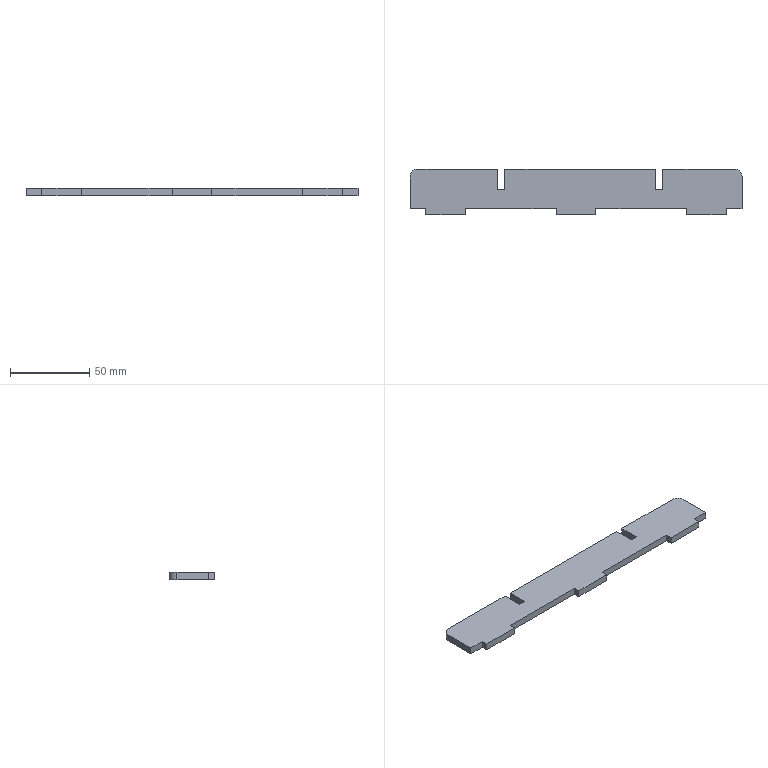Part | SolidWorks | features FlatPattern 1, SMBaseFlange 1, SheetMetal 1 | 1 solid | 28 faces | box 210 x 29 x 4.5 mm | volume 24400 mm3 | plane 26 | cylinder 2 | commonest cylinder face diameters 10 x2
STEP:
#1=CARTESIAN_POINT('',(71.625,-115.747,0.));
#2=VERTEX_POINT('',#1);
#3=CARTESIAN_POINT('',(71.625,-95.747,0.));
#4=VERTEX_POINT('',#3);
#5=CARTESIAN_POINT('',(71.625,-115.747,0.));
#6=DIRECTION('',(0.,1.,0.));
#7=VECTOR('',#6,1000.);
#8=LINE('',#5,#7);
#9=EDGE_CURVE('',#2,#4,#8,.T.);
#10=ORIENTED_EDGE('',*,*,#9,.F.);
#11=CARTESIAN_POINT('',(71.625,-115.747,-4.5));
#12=VERTEX_POINT('',#11);
#13=CARTESIAN_POINT('',(71.625,-115.747,-4.5));
#14=DIRECTION('',(0.,0.,1.));
#15=VECTOR('',#14,1000.);
#16=LINE('',#13,#15);
#17=EDGE_CURVE('',#12,#2,#16,.T.);
#18=ORIENTED_EDGE('',*,*,#17,.F.);
#19=CARTESIAN_POINT('',(71.625,-95.747,-4.5));
#20=VERTEX_POINT('',#19);
#21=CARTESIAN_POINT('',(71.625,-115.747,-4.5));
#22=DIRECTION('',(0.,1.,0.));
#23=VECTOR('',#22,1000.);
#24=LINE('',#21,#23);
#25=EDGE_CURVE('',#12,#20,#24,.T.);
#26=ORIENTED_EDGE('',*,*,#25,.T.);
#27=CARTESIAN_POINT('',(71.625,-95.747,-4.5));
#28=DIRECTION('',(0.,0.,1.));
#29=VECTOR('',#28,1000.);
#30=LINE('',#27,#29);
#31=EDGE_CURVE('',#20,#4,#30,.T.);
#32=ORIENTED_EDGE('',*,*,#31,.T.);
#33=EDGE_LOOP('',(#10,#18,#26,#32));
#34=FACE_OUTER_BOUND('',#33,.T.);
#35=CARTESIAN_POINT('',(71.625,-115.747,-4.5));
#36=DIRECTION('',(1.,0.,0.));
#37=DIRECTION('',(0.,0.,-1.));
#38=AXIS2_PLACEMENT_3D('',#35,#36,#37);
#39=PLANE('',#38);
#40=ADVANCED_FACE('',(#34),#39,.T.);
#41=CARTESIAN_POINT('',(61.625,-115.747,0.));
#42=VERTEX_POINT('',#41);
#43=CARTESIAN_POINT('',(71.625,-115.747,0.));
#44=DIRECTION('',(1.,0.,0.));
#45=VECTOR('',#44,1000.);
#46=LINE('',#43,#45);
#47=EDGE_CURVE('',#42,#2,#46,.T.);
#48=ORIENTED_EDGE('',*,*,#47,.F.);
#49=CARTESIAN_POINT('',(61.625,-115.747,-4.5));
#50=VERTEX_POINT('',#49);
#51=CARTESIAN_POINT('',(61.625,-115.747,-4.5));
#52=DIRECTION('',(0.,0.,1.));
#53=VECTOR('',#52,1000.);
#54=LINE('',#51,#53);
#55=EDGE_CURVE('',#50,#42,#54,.T.);
#56=ORIENTED_EDGE('',*,*,#55,.F.);
#57=CARTESIAN_POINT('',(71.625,-115.747,-4.5));
#58=DIRECTION('',(1.,0.,0.));
#59=VECTOR('',#58,1000.);
#60=LINE('',#57,#59);
#61=EDGE_CURVE('',#50,#12,#60,.T.);
#62=ORIENTED_EDGE('',*,*,#61,.T.);
#63=ORIENTED_EDGE('',*,*,#17,.T.);
#64=EDGE_LOOP('',(#48,#56,#62,#63));
#65=FACE_OUTER_BOUND('',#64,.T.);
#66=CARTESIAN_POINT('',(71.625,-115.747,-4.5));
#67=DIRECTION('',(0.,-1.,0.));
#68=DIRECTION('',(0.,0.,-1.));
#69=AXIS2_PLACEMENT_3D('',#66,#67,#68);
#70=PLANE('',#69);
#71=ADVANCED_FACE('',(#65),#70,.T.);
#72=CARTESIAN_POINT('',(61.625,-119.747,0.));
#73=VERTEX_POINT('',#72);
#74=CARTESIAN_POINT('',(61.625,-115.747,0.));
#75=DIRECTION('',(0.,1.,0.));
#76=VECTOR('',#75,1000.);
#77=LINE('',#74,#76);
#78=EDGE_CURVE('',#73,#42,#77,.T.);
#79=ORIENTED_EDGE('',*,*,#78,.F.);
#80=CARTESIAN_POINT('',(61.625,-119.747,-4.5));
#81=VERTEX_POINT('',#80);
#82=CARTESIAN_POINT('',(61.625,-119.747,-4.5));
#83=DIRECTION('',(0.,0.,1.));
#84=VECTOR('',#83,1000.);
#85=LINE('',#82,#84);
#86=EDGE_CURVE('',#81,#73,#85,.T.);
#87=ORIENTED_EDGE('',*,*,#86,.F.);
#88=CARTESIAN_POINT('',(61.625,-115.747,-4.5));
#89=DIRECTION('',(0.,1.,0.));
#90=VECTOR('',#89,1000.);
#91=LINE('',#88,#90);
#92=EDGE_CURVE('',#81,#50,#91,.T.);
#93=ORIENTED_EDGE('',*,*,#92,.T.);
#94=ORIENTED_EDGE('',*,*,#55,.T.);
#95=EDGE_LOOP('',(#79,#87,#93,#94));
#96=FACE_OUTER_BOUND('',#95,.T.);
#97=CARTESIAN_POINT('',(61.625,-115.747,-4.5));
#98=DIRECTION('',(1.,0.,0.));
#99=DIRECTION('',(0.,0.,-1.));
#100=AXIS2_PLACEMENT_3D('',#97,#98,#99);
#101=PLANE('',#100);
#102=ADVANCED_FACE('',(#96),#101,.T.);
#103=CARTESIAN_POINT('',(36.625,-119.747,0.));
#104=VERTEX_POINT('',#103);
#105=CARTESIAN_POINT('',(61.625,-119.747,0.));
#106=DIRECTION('',(1.,0.,0.));
#107=VECTOR('',#106,1000.);
#108=LINE('',#105,#107);
#109=EDGE_CURVE('',#104,#73,#108,.T.);
#110=ORIENTED_EDGE('',*,*,#109,.F.);
#111=CARTESIAN_POINT('',(36.625,-119.747,-4.5));
#112=VERTEX_POINT('',#111);
#113=CARTESIAN_POINT('',(36.625,-119.747,-4.5));
#114=DIRECTION('',(0.,0.,1.));
#115=VECTOR('',#114,1000.);
#116=LINE('',#113,#115);
#117=EDGE_CURVE('',#112,#104,#116,.T.);
#118=ORIENTED_EDGE('',*,*,#117,.F.);
#119=CARTESIAN_POINT('',(61.625,-119.747,-4.5));
#120=DIRECTION('',(1.,0.,0.));
#121=VECTOR('',#120,1000.);
#122=LINE('',#119,#121);
#123=EDGE_CURVE('',#112,#81,#122,.T.);
#124=ORIENTED_EDGE('',*,*,#123,.T.);
#125=ORIENTED_EDGE('',*,*,#86,.T.);
#126=EDGE_LOOP('',(#110,#118,#124,#125));
#127=FACE_OUTER_BOUND('',#126,.T.);
#128=CARTESIAN_POINT('',(61.625,-119.747,-4.5));
#129=DIRECTION('',(0.,-1.,0.));
#130=DIRECTION('',(1.,0.,0.));
#131=AXIS2_PLACEMENT_3D('',#128,#129,#130);
#132=PLANE('',#131);
#133=ADVANCED_FACE('',(#127),#132,.T.);
#134=CARTESIAN_POINT('',(36.625,-115.747,0.));
#135=VERTEX_POINT('',#134);
#136=CARTESIAN_POINT('',(36.625,-119.747,0.));
#137=DIRECTION('',(0.,-1.,0.));
#138=VECTOR('',#137,1000.);
#139=LINE('',#136,#138);
#140=EDGE_CURVE('',#135,#104,#139,.T.);
#141=ORIENTED_EDGE('',*,*,#140,.F.);
#142=CARTESIAN_POINT('',(36.625,-115.747,-4.5));
#143=VERTEX_POINT('',#142);
#144=CARTESIAN_POINT('',(36.625,-115.747,-4.5));
#145=DIRECTION('',(0.,0.,1.));
#146=VECTOR('',#145,1000.);
#147=LINE('',#144,#146);
#148=EDGE_CURVE('',#143,#135,#147,.T.);
#149=ORIENTED_EDGE('',*,*,#148,.F.);
#150=CARTESIAN_POINT('',(36.625,-119.747,-4.5));
#151=DIRECTION('',(0.,-1.,0.));
#152=VECTOR('',#151,1000.);
#153=LINE('',#150,#152);
#154=EDGE_CURVE('',#143,#112,#153,.T.);
#155=ORIENTED_EDGE('',*,*,#154,.T.);
#156=ORIENTED_EDGE('',*,*,#117,.T.);
#157=EDGE_LOOP('',(#141,#149,#155,#156));
#158=FACE_OUTER_BOUND('',#157,.T.);
#159=CARTESIAN_POINT('',(36.625,-119.747,-4.5));
#160=DIRECTION('',(-1.,0.,0.));
#161=DIRECTION('',(0.,0.,1.));
#162=AXIS2_PLACEMENT_3D('',#159,#160,#161);
#163=PLANE('',#162);
#164=ADVANCED_FACE('',(#158),#163,.T.);
#165=CARTESIAN_POINT('',(-20.875,-115.747,0.));
#166=VERTEX_POINT('',#165);
#167=CARTESIAN_POINT('',(36.625,-115.747,0.));
#168=DIRECTION('',(1.,0.,0.));
#169=VECTOR('',#168,1000.);
#170=LINE('',#167,#169);
#171=EDGE_CURVE('',#166,#135,#170,.T.);
#172=ORIENTED_EDGE('',*,*,#171,.F.);
#173=CARTESIAN_POINT('',(-20.875,-115.747,-4.5));
#174=VERTEX_POINT('',#173);
#175=CARTESIAN_POINT('',(-20.875,-115.747,-4.5));
#176=DIRECTION('',(0.,0.,1.));
#177=VECTOR('',#176,1000.);
#178=LINE('',#175,#177);
#179=EDGE_CURVE('',#174,#166,#178,.T.);
#180=ORIENTED_EDGE('',*,*,#179,.F.);
#181=CARTESIAN_POINT('',(36.625,-115.747,-4.5));
#182=DIRECTION('',(1.,0.,0.));
#183=VECTOR('',#182,1000.);
#184=LINE('',#181,#183);
#185=EDGE_CURVE('',#174,#143,#184,.T.);
#186=ORIENTED_EDGE('',*,*,#185,.T.);
#187=ORIENTED_EDGE('',*,*,#148,.T.);
#188=EDGE_LOOP('',(#172,#180,#186,#187));
#189=FACE_OUTER_BOUND('',#188,.T.);
#190=CARTESIAN_POINT('',(36.625,-115.747,-4.5));
#191=DIRECTION('',(0.,-1.,0.));
#192=DIRECTION('',(1.,0.,0.));
#193=AXIS2_PLACEMENT_3D('',#190,#191,#192);
#194=PLANE('',#193);
#195=ADVANCED_FACE('',(#189),#194,.T.);
#196=CARTESIAN_POINT('',(-20.875,-119.747,0.));
#197=VERTEX_POINT('',#196);
#198=CARTESIAN_POINT('',(-20.875,-115.747,0.));
#199=DIRECTION('',(0.,1.,0.));
#200=VECTOR('',#199,1000.);
#201=LINE('',#198,#200);
#202=EDGE_CURVE('',#197,#166,#201,.T.);
#203=ORIENTED_EDGE('',*,*,#202,.F.);
#204=CARTESIAN_POINT('',(-20.875,-119.747,-4.5));
#205=VERTEX_POINT('',#204);
#206=CARTESIAN_POINT('',(-20.875,-119.747,-4.5));
#207=DIRECTION('',(0.,0.,1.));
#208=VECTOR('',#207,1000.);
#209=LINE('',#206,#208);
#210=EDGE_CURVE('',#205,#197,#209,.T.);
#211=ORIENTED_EDGE('',*,*,#210,.F.);
#212=CARTESIAN_POINT('',(-20.875,-115.747,-4.5));
#213=DIRECTION('',(0.,1.,0.));
#214=VECTOR('',#213,1000.);
#215=LINE('',#212,#214);
#216=EDGE_CURVE('',#205,#174,#215,.T.);
#217=ORIENTED_EDGE('',*,*,#216,.T.);
#218=ORIENTED_EDGE('',*,*,#179,.T.);
#219=EDGE_LOOP('',(#203,#211,#217,#218));
#220=FACE_OUTER_BOUND('',#219,.T.);
#221=CARTESIAN_POINT('',(-20.875,-115.747,-4.5));
#222=DIRECTION('',(1.,0.,0.));
#223=DIRECTION('',(0.,1.,0.));
#224=AXIS2_PLACEMENT_3D('',#221,#222,#223);
#225=PLANE('',#224);
#226=ADVANCED_FACE('',(#220),#225,.T.);
#227=CARTESIAN_POINT('',(-45.875,-119.747,0.));
#228=VERTEX_POINT('',#227);
#229=CARTESIAN_POINT('',(-20.875,-119.747,0.));
#230=DIRECTION('',(1.,0.,0.));
#231=VECTOR('',#230,1000.);
#232=LINE('',#229,#231);
#233=EDGE_CURVE('',#228,#197,#232,.T.);
#234=ORIENTED_EDGE('',*,*,#233,.F.);
#235=CARTESIAN_POINT('',(-45.875,-119.747,-4.5));
#236=VERTEX_POINT('',#235);
#237=CARTESIAN_POINT('',(-45.875,-119.747,-4.5));
#238=DIRECTION('',(0.,0.,1.));
#239=VECTOR('',#238,1000.);
#240=LINE('',#237,#239);
#241=EDGE_CURVE('',#236,#228,#240,.T.);
#242=ORIENTED_EDGE('',*,*,#241,.F.);
#243=CARTESIAN_POINT('',(-20.875,-119.747,-4.5));
#244=DIRECTION('',(1.,0.,0.));
#245=VECTOR('',#244,1000.);
#246=LINE('',#243,#245);
#247=EDGE_CURVE('',#236,#205,#246,.T.);
#248=ORIENTED_EDGE('',*,*,#247,.T.);
#249=ORIENTED_EDGE('',*,*,#210,.T.);
#250=EDGE_LOOP('',(#234,#242,#248,#249));
#251=FACE_OUTER_BOUND('',#250,.T.);
#252=CARTESIAN_POINT('',(-20.875,-119.747,-4.5));
#253=DIRECTION('',(0.,-1.,0.));
#254=DIRECTION('',(0.,0.,-1.));
#255=AXIS2_PLACEMENT_3D('',#252,#253,#254);
#256=PLANE('',#255);
#257=ADVANCED_FACE('',(#251),#256,.T.);
#258=CARTESIAN_POINT('',(-45.875,-115.747,0.));
#259=VERTEX_POINT('',#258);
#260=CARTESIAN_POINT('',(-45.875,-119.747,0.));
#261=DIRECTION('',(0.,-1.,0.));
#262=VECTOR('',#261,1000.);
#263=LINE('',#260,#262);
#264=EDGE_CURVE('',#259,#228,#263,.T.);
#265=ORIENTED_EDGE('',*,*,#264,.F.);
#266=CARTESIAN_POINT('',(-45.875,-115.747,-4.5));
#267=VERTEX_POINT('',#266);
#268=CARTESIAN_POINT('',(-45.875,-115.747,-4.5));
#269=DIRECTION('',(0.,0.,1.));
#270=VECTOR('',#269,1000.);
#271=LINE('',#268,#270);
#272=EDGE_CURVE('',#267,#259,#271,.T.);
#273=ORIENTED_EDGE('',*,*,#272,.F.);
#274=CARTESIAN_POINT('',(-45.875,-119.747,-4.5));
#275=DIRECTION('',(0.,-1.,0.));
#276=VECTOR('',#275,1000.);
#277=LINE('',#274,#276);
#278=EDGE_CURVE('',#267,#236,#277,.T.);
#279=ORIENTED_EDGE('',*,*,#278,.T.);
#280=ORIENTED_EDGE('',*,*,#241,.T.);
#281=EDGE_LOOP('',(#265,#273,#279,#280));
#282=FACE_OUTER_BOUND('',#281,.T.);
#283=CARTESIAN_POINT('',(-45.875,-119.747,-4.5));
#284=DIRECTION('',(-1.,0.,0.));
#285=DIRECTION('',(0.,0.,1.));
#286=AXIS2_PLACEMENT_3D('',#283,#284,#285);
#287=PLANE('',#286);
#288=ADVANCED_FACE('',(#282),#287,.T.);
#289=CARTESIAN_POINT('',(-103.375,-115.747,0.));
#290=VERTEX_POINT('',#289);
#291=CARTESIAN_POINT('',(-45.875,-115.747,0.));
#292=DIRECTION('',(1.,0.,0.));
#293=VECTOR('',#292,1000.);
#294=LINE('',#291,#293);
#295=EDGE_CURVE('',#290,#259,#294,.T.);
#296=ORIENTED_EDGE('',*,*,#295,.F.);
#297=CARTESIAN_POINT('',(-103.375,-115.747,-4.5));
#298=VERTEX_POINT('',#297);
#299=CARTESIAN_POINT('',(-103.375,-115.747,-4.5));
#300=DIRECTION('',(0.,0.,1.));
#301=VECTOR('',#300,1000.);
#302=LINE('',#299,#301);
#303=EDGE_CURVE('',#298,#290,#302,.T.);
#304=ORIENTED_EDGE('',*,*,#303,.F.);
#305=CARTESIAN_POINT('',(-45.875,-115.747,-4.5));
#306=DIRECTION('',(1.,0.,0.));
#307=VECTOR('',#306,1000.);
#308=LINE('',#305,#307);
#309=EDGE_CURVE('',#298,#267,#308,.T.);
#310=ORIENTED_EDGE('',*,*,#309,.T.);
#311=ORIENTED_EDGE('',*,*,#272,.T.);
#312=EDGE_LOOP('',(#296,#304,#310,#311));
#313=FACE_OUTER_BOUND('',#312,.T.);
#314=CARTESIAN_POINT('',(-45.875,-115.747,-4.5));
#315=DIRECTION('',(0.,-1.,0.));
#316=DIRECTION('',(1.,0.,0.));
#317=AXIS2_PLACEMENT_3D('',#314,#315,#316);
#318=PLANE('',#317);
#319=ADVANCED_FACE('',(#313),#318,.T.);
#320=CARTESIAN_POINT('',(-103.375,-119.747,0.));
#321=VERTEX_POINT('',#320);
#322=CARTESIAN_POINT('',(-103.375,-115.747,0.));
#323=DIRECTION('',(0.,1.,0.));
#324=VECTOR('',#323,1000.);
#325=LINE('',#322,#324);
#326=EDGE_CURVE('',#321,#290,#325,.T.);
#327=ORIENTED_EDGE('',*,*,#326,.F.);
#328=CARTESIAN_POINT('',(-103.375,-119.747,-4.5));
#329=VERTEX_POINT('',#328);
#330=CARTESIAN_POINT('',(-103.375,-119.747,-4.5));
#331=DIRECTION('',(0.,0.,1.));
#332=VECTOR('',#331,1000.);
#333=LINE('',#330,#332);
#334=EDGE_CURVE('',#329,#321,#333,.T.);
#335=ORIENTED_EDGE('',*,*,#334,.F.);
#336=CARTESIAN_POINT('',(-103.375,-115.747,-4.5));
#337=DIRECTION('',(0.,1.,0.));
#338=VECTOR('',#337,1000.);
#339=LINE('',#336,#338);
#340=EDGE_CURVE('',#329,#298,#339,.T.);
#341=ORIENTED_EDGE('',*,*,#340,.T.);
#342=ORIENTED_EDGE('',*,*,#303,.T.);
#343=EDGE_LOOP('',(#327,#335,#341,#342));
#344=FACE_OUTER_BOUND('',#343,.T.);
#345=CARTESIAN_POINT('',(-103.375,-115.747,-4.5));
#346=DIRECTION('',(1.,0.,0.));
#347=DIRECTION('',(0.,0.,-1.));
#348=AXIS2_PLACEMENT_3D('',#345,#346,#347);
#349=PLANE('',#348);
#350=ADVANCED_FACE('',(#344),#349,.T.);
#351=CARTESIAN_POINT('',(-128.375,-119.747,0.));
#352=VERTEX_POINT('',#351);
#353=CARTESIAN_POINT('',(-103.375,-119.747,0.));
#354=DIRECTION('',(1.,0.,0.));
#355=VECTOR('',#354,1000.);
#356=LINE('',#353,#355);
#357=EDGE_CURVE('',#352,#321,#356,.T.);
#358=ORIENTED_EDGE('',*,*,#357,.F.);
#359=CARTESIAN_POINT('',(-128.375,-119.747,-4.5));
#360=VERTEX_POINT('',#359);
#361=CARTESIAN_POINT('',(-128.375,-119.747,-4.5));
#362=DIRECTION('',(0.,0.,1.));
#363=VECTOR('',#362,1000.);
#364=LINE('',#361,#363);
#365=EDGE_CURVE('',#360,#352,#364,.T.);
#366=ORIENTED_EDGE('',*,*,#365,.F.);
#367=CARTESIAN_POINT('',(-103.375,-119.747,-4.5));
#368=DIRECTION('',(1.,0.,0.));
#369=VECTOR('',#368,1000.);
#370=LINE('',#367,#369);
#371=EDGE_CURVE('',#360,#329,#370,.T.);
#372=ORIENTED_EDGE('',*,*,#371,.T.);
#373=ORIENTED_EDGE('',*,*,#334,.T.);
#374=EDGE_LOOP('',(#358,#366,#372,#373));
#375=FACE_OUTER_BOUND('',#374,.T.);
#376=CARTESIAN_POINT('',(-103.375,-119.747,-4.5));
#377=DIRECTION('',(0.,-1.,0.));
#378=DIRECTION('',(1.,0.,0.));
#379=AXIS2_PLACEMENT_3D('',#376,#377,#378);
#380=PLANE('',#379);
#381=ADVANCED_FACE('',(#375),#380,.T.);
#382=CARTESIAN_POINT('',(-128.375,-115.747,0.));
#383=VERTEX_POINT('',#382);
#384=CARTESIAN_POINT('',(-128.375,-119.747,0.));
#385=DIRECTION('',(0.,-1.,0.));
#386=VECTOR('',#385,1000.);
#387=LINE('',#384,#386);
#388=EDGE_CURVE('',#383,#352,#387,.T.);
#389=ORIENTED_EDGE('',*,*,#388,.F.);
#390=CARTESIAN_POINT('',(-128.375,-115.747,-4.5));
#391=VERTEX_POINT('',#390);
#392=CARTESIAN_POINT('',(-128.375,-115.747,-4.5));
#393=DIRECTION('',(0.,0.,1.));
#394=VECTOR('',#393,1000.);
#395=LINE('',#392,#394);
#396=EDGE_CURVE('',#391,#383,#395,.T.);
#397=ORIENTED_EDGE('',*,*,#396,.F.);
#398=CARTESIAN_POINT('',(-128.375,-119.747,-4.5));
#399=DIRECTION('',(0.,-1.,0.));
#400=VECTOR('',#399,1000.);
#401=LINE('',#398,#400);
#402=EDGE_CURVE('',#391,#360,#401,.T.);
#403=ORIENTED_EDGE('',*,*,#402,.T.);
#404=ORIENTED_EDGE('',*,*,#365,.T.);
#405=EDGE_LOOP('',(#389,#397,#403,#404));
#406=FACE_OUTER_BOUND('',#405,.T.);
#407=CARTESIAN_POINT('',(-128.375,-119.747,-4.5));
#408=DIRECTION('',(-1.,0.,0.));
#409=DIRECTION('',(0.,0.,1.));
#410=AXIS2_PLACEMENT_3D('',#407,#408,#409);
#411=PLANE('',#410);
#412=ADVANCED_FACE('',(#406),#411,.T.);
#413=CARTESIAN_POINT('',(-138.375,-115.747,0.));
#414=VERTEX_POINT('',#413);
#415=CARTESIAN_POINT('',(-128.375,-115.747,0.));
#416=DIRECTION('',(1.,0.,0.));
#417=VECTOR('',#416,1000.);
#418=LINE('',#415,#417);
#419=EDGE_CURVE('',#414,#383,#418,.T.);
#420=ORIENTED_EDGE('',*,*,#419,.F.);
#421=CARTESIAN_POINT('',(-138.375,-115.747,-4.5));
#422=VERTEX_POINT('',#421);
#423=CARTESIAN_POINT('',(-138.375,-115.747,-4.5));
#424=DIRECTION('',(0.,0.,1.));
#425=VECTOR('',#424,1000.);
#426=LINE('',#423,#425);
#427=EDGE_CURVE('',#422,#414,#426,.T.);
#428=ORIENTED_EDGE('',*,*,#427,.F.);
#429=CARTESIAN_POINT('',(-128.375,-115.747,-4.5));
#430=DIRECTION('',(1.,0.,0.));
#431=VECTOR('',#430,1000.);
#432=LINE('',#429,#431);
#433=EDGE_CURVE('',#422,#391,#432,.T.);
#434=ORIENTED_EDGE('',*,*,#433,.T.);
#435=ORIENTED_EDGE('',*,*,#396,.T.);
#436=EDGE_LOOP('',(#420,#428,#434,#435));
#437=FACE_OUTER_BOUND('',#436,.T.);
#438=CARTESIAN_POINT('',(-128.375,-115.747,-4.5));
#439=DIRECTION('',(0.,-1.,0.));
#440=DIRECTION('',(1.,0.,0.));
#441=AXIS2_PLACEMENT_3D('',#438,#439,#440);
#442=PLANE('',#441);
#443=ADVANCED_FACE('',(#437),#442,.T.);
#444=CARTESIAN_POINT('',(-138.375,-95.747,0.));
#445=VERTEX_POINT('',#444);
#446=CARTESIAN_POINT('',(-138.375,-115.747,0.));
#447=DIRECTION('',(0.,-1.,0.));
#448=VECTOR('',#447,1000.);
#449=LINE('',#446,#448);
#450=EDGE_CURVE('',#445,#414,#449,.T.);
#451=ORIENTED_EDGE('',*,*,#450,.F.);
#452=CARTESIAN_POINT('',(-138.375,-95.747,-4.5));
#453=VERTEX_POINT('',#452);
#454=CARTESIAN_POINT('',(-138.375,-95.747,-4.5));
#455=DIRECTION('',(0.,0.,1.));
#456=VECTOR('',#455,1000.);
#457=LINE('',#454,#456);
#458=EDGE_CURVE('',#453,#445,#457,.T.);
#459=ORIENTED_EDGE('',*,*,#458,.F.);
#460=CARTESIAN_POINT('',(-138.375,-115.747,-4.5));
#461=DIRECTION('',(0.,-1.,0.));
#462=VECTOR('',#461,1000.);
#463=LINE('',#460,#462);
#464=EDGE_CURVE('',#453,#422,#463,.T.);
#465=ORIENTED_EDGE('',*,*,#464,.T.);
#466=ORIENTED_EDGE('',*,*,#427,.T.);
#467=EDGE_LOOP('',(#451,#459,#465,#466));
#468=FACE_OUTER_BOUND('',#467,.T.);
#469=CARTESIAN_POINT('',(-138.375,-115.747,-4.5));
#470=DIRECTION('',(-1.,0.,0.));
#471=DIRECTION('',(0.,0.,1.));
#472=AXIS2_PLACEMENT_3D('',#469,#470,#471);
#473=PLANE('',#472);
#474=ADVANCED_FACE('',(#468),#473,.T.);
#475=CARTESIAN_POINT('',(-133.375,-90.747,0.));
#476=VERTEX_POINT('',#475);
#477=CARTESIAN_POINT('',(-133.375,-95.747,0.));
#478=DIRECTION('',(0.,0.,1.));
#479=DIRECTION('',(1.,0.,0.));
#480=AXIS2_PLACEMENT_3D('',#477,#478,#479);
#481=CIRCLE('',#480,5.);
#482=EDGE_CURVE('',#476,#445,#481,.T.);
#483=ORIENTED_EDGE('',*,*,#482,.F.);
#484=CARTESIAN_POINT('',(-133.375,-90.747,-4.5));
#485=VERTEX_POINT('',#484);
#486=CARTESIAN_POINT('',(-133.375,-90.747,-4.5));
#487=DIRECTION('',(0.,0.,1.));
#488=VECTOR('',#487,1000.);
#489=LINE('',#486,#488);
#490=EDGE_CURVE('',#485,#476,#489,.T.);
#491=ORIENTED_EDGE('',*,*,#490,.F.);
#492=CARTESIAN_POINT('',(-133.375,-95.747,-4.5));
#493=DIRECTION('',(0.,0.,1.));
#494=DIRECTION('',(1.,0.,0.));
#495=AXIS2_PLACEMENT_3D('',#492,#493,#494);
#496=CIRCLE('',#495,5.);
#497=EDGE_CURVE('',#485,#453,#496,.T.);
#498=ORIENTED_EDGE('',*,*,#497,.T.);
#499=ORIENTED_EDGE('',*,*,#458,.T.);
#500=EDGE_LOOP('',(#483,#491,#498,#499));
#501=FACE_OUTER_BOUND('',#500,.T.);
#502=CARTESIAN_POINT('',(-133.375,-95.747,-4.5));
#503=DIRECTION('',(0.,0.,1.));
#504=DIRECTION('',(1.,0.,0.));
#505=AXIS2_PLACEMENT_3D('',#502,#503,#504);
#506=CYLINDRICAL_SURFACE('',#505,5.);
#507=ADVANCED_FACE('',(#501),#506,.T.);
#508=CARTESIAN_POINT('',(-82.875,-90.747,0.));
#509=VERTEX_POINT('',#508);
#510=CARTESIAN_POINT('',(-82.875,-90.747,0.));
#511=DIRECTION('',(-1.,0.,0.));
#512=VECTOR('',#511,1000.);
#513=LINE('',#510,#512);
#514=EDGE_CURVE('',#509,#476,#513,.T.);
#515=ORIENTED_EDGE('',*,*,#514,.F.);
#516=CARTESIAN_POINT('',(-82.875,-90.747,-4.5));
#517=VERTEX_POINT('',#516);
#518=CARTESIAN_POINT('',(-82.875,-90.747,-4.5));
#519=DIRECTION('',(0.,0.,1.));
#520=VECTOR('',#519,1000.);
#521=LINE('',#518,#520);
#522=EDGE_CURVE('',#517,#509,#521,.T.);
#523=ORIENTED_EDGE('',*,*,#522,.F.);
#524=CARTESIAN_POINT('',(-82.875,-90.747,-4.5));
#525=DIRECTION('',(-1.,0.,0.));
#526=VECTOR('',#525,1000.);
#527=LINE('',#524,#526);
#528=EDGE_CURVE('',#517,#485,#527,.T.);
#529=ORIENTED_EDGE('',*,*,#528,.T.);
#530=ORIENTED_EDGE('',*,*,#490,.T.);
#531=EDGE_LOOP('',(#515,#523,#529,#530));
#532=FACE_OUTER_BOUND('',#531,.T.);
#533=CARTESIAN_POINT('',(-82.875,-90.747,-4.5));
#534=DIRECTION('',(0.,1.,0.));
#535=DIRECTION('',(-1.,0.,0.));
#536=AXIS2_PLACEMENT_3D('',#533,#534,#535);
#537=PLANE('',#536);
#538=ADVANCED_FACE('',(#532),#537,.T.);
#539=CARTESIAN_POINT('',(-82.875,-103.747,0.));
#540=VERTEX_POINT('',#539);
#541=CARTESIAN_POINT('',(-82.875,-103.747,0.));
#542=DIRECTION('',(0.,1.,0.));
#543=VECTOR('',#542,1000.);
#544=LINE('',#541,#543);
#545=EDGE_CURVE('',#540,#509,#544,.T.);
#546=ORIENTED_EDGE('',*,*,#545,.F.);
#547=CARTESIAN_POINT('',(-82.875,-103.747,-4.5));
#548=VERTEX_POINT('',#547);
#549=CARTESIAN_POINT('',(-82.875,-103.747,-4.5));
#550=DIRECTION('',(0.,0.,1.));
#551=VECTOR('',#550,1000.);
#552=LINE('',#549,#551);
#553=EDGE_CURVE('',#548,#540,#552,.T.);
#554=ORIENTED_EDGE('',*,*,#553,.F.);
#555=CARTESIAN_POINT('',(-82.875,-103.747,-4.5));
#556=DIRECTION('',(0.,1.,0.));
#557=VECTOR('',#556,1000.);
#558=LINE('',#555,#557);
#559=EDGE_CURVE('',#548,#517,#558,.T.);
#560=ORIENTED_EDGE('',*,*,#559,.T.);
#561=ORIENTED_EDGE('',*,*,#522,.T.);
#562=EDGE_LOOP('',(#546,#554,#560,#561));
#563=FACE_OUTER_BOUND('',#562,.T.);
#564=CARTESIAN_POINT('',(-82.875,-103.747,-4.5));
#565=DIRECTION('',(1.,0.,0.));
#566=DIRECTION('',(0.,1.,0.));
#567=AXIS2_PLACEMENT_3D('',#564,#565,#566);
#568=PLANE('',#567);
#569=ADVANCED_FACE('',(#563),#568,.T.);
#570=CARTESIAN_POINT('',(-78.375,-103.747,0.));
#571=VERTEX_POINT('',#570);
#572=CARTESIAN_POINT('',(-78.375,-103.747,0.));
#573=DIRECTION('',(-1.,0.,0.));
#574=VECTOR('',#573,1000.);
#575=LINE('',#572,#574);
#576=EDGE_CURVE('',#571,#540,#575,.T.);
#577=ORIENTED_EDGE('',*,*,#576,.F.);
#578=CARTESIAN_POINT('',(-78.375,-103.747,-4.5));
#579=VERTEX_POINT('',#578);
#580=CARTESIAN_POINT('',(-78.375,-103.747,-4.5));
#581=DIRECTION('',(0.,0.,1.));
#582=VECTOR('',#581,1000.);
#583=LINE('',#580,#582);
#584=EDGE_CURVE('',#579,#571,#583,.T.);
#585=ORIENTED_EDGE('',*,*,#584,.F.);
#586=CARTESIAN_POINT('',(-78.375,-103.747,-4.5));
#587=DIRECTION('',(-1.,0.,0.));
#588=VECTOR('',#587,1000.);
#589=LINE('',#586,#588);
#590=EDGE_CURVE('',#579,#548,#589,.T.);
#591=ORIENTED_EDGE('',*,*,#590,.T.);
#592=ORIENTED_EDGE('',*,*,#553,.T.);
#593=EDGE_LOOP('',(#577,#585,#591,#592));
#594=FACE_OUTER_BOUND('',#593,.T.);
#595=CARTESIAN_POINT('',(-78.375,-103.747,-4.5));
#596=DIRECTION('',(0.,1.,0.));
#597=DIRECTION('',(0.,0.,1.));
#598=AXIS2_PLACEMENT_3D('',#595,#596,#597);
#599=PLANE('',#598);
#600=ADVANCED_FACE('',(#594),#599,.T.);
#601=CARTESIAN_POINT('',(-78.375,-90.747,0.));
#602=VERTEX_POINT('',#601);
#603=CARTESIAN_POINT('',(-78.375,-90.747,0.));
#604=DIRECTION('',(0.,-1.,0.));
#605=VECTOR('',#604,1000.);
#606=LINE('',#603,#605);
#607=EDGE_CURVE('',#602,#571,#606,.T.);
#608=ORIENTED_EDGE('',*,*,#607,.F.);
#609=CARTESIAN_POINT('',(-78.375,-90.747,-4.5));
#610=VERTEX_POINT('',#609);
#611=CARTESIAN_POINT('',(-78.375,-90.747,-4.5));
#612=DIRECTION('',(0.,0.,1.));
#613=VECTOR('',#612,1000.);
#614=LINE('',#611,#613);
#615=EDGE_CURVE('',#610,#602,#614,.T.);
#616=ORIENTED_EDGE('',*,*,#615,.F.);
#617=CARTESIAN_POINT('',(-78.375,-90.747,-4.5));
#618=DIRECTION('',(0.,-1.,0.));
#619=VECTOR('',#618,1000.);
#620=LINE('',#617,#619);
#621=EDGE_CURVE('',#610,#579,#620,.T.);
#622=ORIENTED_EDGE('',*,*,#621,.T.);
#623=ORIENTED_EDGE('',*,*,#584,.T.);
#624=EDGE_LOOP('',(#608,#616,#622,#623));
#625=FACE_OUTER_BOUND('',#624,.T.);
#626=CARTESIAN_POINT('',(-78.375,-90.747,-4.5));
#627=DIRECTION('',(-1.,0.,0.));
#628=DIRECTION('',(0.,-1.,0.));
#629=AXIS2_PLACEMENT_3D('',#626,#627,#628);
#630=PLANE('',#629);
#631=ADVANCED_FACE('',(#625),#630,.T.);
#632=CARTESIAN_POINT('',(17.125,-90.747,0.));
#633=VERTEX_POINT('',#632);
#634=CARTESIAN_POINT('',(17.125,-90.747,0.));
#635=DIRECTION('',(-1.,0.,0.));
#636=VECTOR('',#635,1000.);
#637=LINE('',#634,#636);
#638=EDGE_CURVE('',#633,#602,#637,.T.);
#639=ORIENTED_EDGE('',*,*,#638,.F.);
#640=CARTESIAN_POINT('',(17.125,-90.747,-4.5));
#641=VERTEX_POINT('',#640);
#642=CARTESIAN_POINT('',(17.125,-90.747,-4.5));
#643=DIRECTION('',(0.,0.,1.));
#644=VECTOR('',#643,1000.);
#645=LINE('',#642,#644);
#646=EDGE_CURVE('',#641,#633,#645,.T.);
#647=ORIENTED_EDGE('',*,*,#646,.F.);
#648=CARTESIAN_POINT('',(17.125,-90.747,-4.5));
#649=DIRECTION('',(-1.,0.,0.));
#650=VECTOR('',#649,1000.);
#651=LINE('',#648,#650);
#652=EDGE_CURVE('',#641,#610,#651,.T.);
#653=ORIENTED_EDGE('',*,*,#652,.T.);
#654=ORIENTED_EDGE('',*,*,#615,.T.);
#655=EDGE_LOOP('',(#639,#647,#653,#654));
#656=FACE_OUTER_BOUND('',#655,.T.);
#657=CARTESIAN_POINT('',(17.125,-90.747,-4.5));
#658=DIRECTION('',(0.,1.,0.));
#659=DIRECTION('',(-1.,0.,0.));
#660=AXIS2_PLACEMENT_3D('',#657,#658,#659);
#661=PLANE('',#660);
#662=ADVANCED_FACE('',(#656),#661,.T.);
#663=CARTESIAN_POINT('',(17.125,-103.747,0.));
#664=VERTEX_POINT('',#663);
#665=CARTESIAN_POINT('',(17.125,-103.747,0.));
#666=DIRECTION('',(0.,1.,0.));
#667=VECTOR('',#666,1000.);
#668=LINE('',#665,#667);
#669=EDGE_CURVE('',#664,#633,#668,.T.);
#670=ORIENTED_EDGE('',*,*,#669,.F.);
#671=CARTESIAN_POINT('',(17.125,-103.747,-4.5));
#672=VERTEX_POINT('',#671);
#673=CARTESIAN_POINT('',(17.125,-103.747,-4.5));
#674=DIRECTION('',(0.,0.,1.));
#675=VECTOR('',#674,1000.);
#676=LINE('',#673,#675);
#677=EDGE_CURVE('',#672,#664,#676,.T.);
#678=ORIENTED_EDGE('',*,*,#677,.F.);
#679=CARTESIAN_POINT('',(17.125,-103.747,-4.5));
#680=DIRECTION('',(0.,1.,0.));
#681=VECTOR('',#680,1000.);
#682=LINE('',#679,#681);
#683=EDGE_CURVE('',#672,#641,#682,.T.);
#684=ORIENTED_EDGE('',*,*,#683,.T.);
#685=ORIENTED_EDGE('',*,*,#646,.T.);
#686=EDGE_LOOP('',(#670,#678,#684,#685));
#687=FACE_OUTER_BOUND('',#686,.T.);
#688=CARTESIAN_POINT('',(17.125,-103.747,-4.5));
#689=DIRECTION('',(1.,0.,0.));
#690=DIRECTION('',(0.,1.,0.));
#691=AXIS2_PLACEMENT_3D('',#688,#689,#690);
#692=PLANE('',#691);
#693=ADVANCED_FACE('',(#687),#692,.T.);
#694=CARTESIAN_POINT('',(21.625,-103.747,0.));
#695=VERTEX_POINT('',#694);
#696=CARTESIAN_POINT('',(21.625,-103.747,0.));
#697=DIRECTION('',(-1.,0.,0.));
#698=VECTOR('',#697,1000.);
#699=LINE('',#696,#698);
#700=EDGE_CURVE('',#695,#664,#699,.T.);
#701=ORIENTED_EDGE('',*,*,#700,.F.);
#702=CARTESIAN_POINT('',(21.625,-103.747,-4.5));
#703=VERTEX_POINT('',#702);
#704=CARTESIAN_POINT('',(21.625,-103.747,-4.5));
#705=DIRECTION('',(0.,0.,1.));
#706=VECTOR('',#705,1000.);
#707=LINE('',#704,#706);
#708=EDGE_CURVE('',#703,#695,#707,.T.);
#709=ORIENTED_EDGE('',*,*,#708,.F.);
#710=CARTESIAN_POINT('',(21.625,-103.747,-4.5));
#711=DIRECTION('',(-1.,0.,0.));
#712=VECTOR('',#711,1000.);
#713=LINE('',#710,#712);
#714=EDGE_CURVE('',#703,#672,#713,.T.);
#715=ORIENTED_EDGE('',*,*,#714,.T.);
#716=ORIENTED_EDGE('',*,*,#677,.T.);
#717=EDGE_LOOP('',(#701,#709,#715,#716));
#718=FACE_OUTER_BOUND('',#717,.T.);
#719=CARTESIAN_POINT('',(21.625,-103.747,-4.5));
#720=DIRECTION('',(0.,1.,0.));
#721=DIRECTION('',(0.,0.,1.));
#722=AXIS2_PLACEMENT_3D('',#719,#720,#721);
#723=PLANE('',#722);
#724=ADVANCED_FACE('',(#718),#723,.T.);
#725=CARTESIAN_POINT('',(21.625,-90.747,0.));
#726=VERTEX_POINT('',#725);
#727=CARTESIAN_POINT('',(21.625,-90.747,0.));
#728=DIRECTION('',(0.,-1.,0.));
#729=VECTOR('',#728,1000.);
#730=LINE('',#727,#729);
#731=EDGE_CURVE('',#726,#695,#730,.T.);
#732=ORIENTED_EDGE('',*,*,#731,.F.);
#733=CARTESIAN_POINT('',(21.625,-90.747,-4.5));
#734=VERTEX_POINT('',#733);
#735=CARTESIAN_POINT('',(21.625,-90.747,-4.5));
#736=DIRECTION('',(0.,0.,1.));
#737=VECTOR('',#736,1000.);
#738=LINE('',#735,#737);
#739=EDGE_CURVE('',#734,#726,#738,.T.);
#740=ORIENTED_EDGE('',*,*,#739,.F.);
#741=CARTESIAN_POINT('',(21.625,-90.747,-4.5));
#742=DIRECTION('',(0.,-1.,0.));
#743=VECTOR('',#742,1000.);
#744=LINE('',#741,#743);
#745=EDGE_CURVE('',#734,#703,#744,.T.);
#746=ORIENTED_EDGE('',*,*,#745,.T.);
#747=ORIENTED_EDGE('',*,*,#708,.T.);
#748=EDGE_LOOP('',(#732,#740,#746,#747));
#749=FACE_OUTER_BOUND('',#748,.T.);
#750=CARTESIAN_POINT('',(21.625,-90.747,-4.5));
#751=DIRECTION('',(-1.,0.,0.));
#752=DIRECTION('',(0.,-1.,0.));
#753=AXIS2_PLACEMENT_3D('',#750,#751,#752);
#754=PLANE('',#753);
#755=ADVANCED_FACE('',(#749),#754,.T.);
#756=CARTESIAN_POINT('',(66.625,-90.747,0.));
#757=VERTEX_POINT('',#756);
#758=CARTESIAN_POINT('',(66.625,-90.747,0.));
#759=DIRECTION('',(-1.,0.,0.));
#760=VECTOR('',#759,1000.);
#761=LINE('',#758,#760);
#762=EDGE_CURVE('',#757,#726,#761,.T.);
#763=ORIENTED_EDGE('',*,*,#762,.F.);
#764=CARTESIAN_POINT('',(66.625,-90.747,-4.5));
#765=VERTEX_POINT('',#764);
#766=CARTESIAN_POINT('',(66.625,-90.747,-4.5));
#767=DIRECTION('',(0.,0.,1.));
#768=VECTOR('',#767,1000.);
#769=LINE('',#766,#768);
#770=EDGE_CURVE('',#765,#757,#769,.T.);
#771=ORIENTED_EDGE('',*,*,#770,.F.);
#772=CARTESIAN_POINT('',(66.625,-90.747,-4.5));
#773=DIRECTION('',(-1.,0.,0.));
#774=VECTOR('',#773,1000.);
#775=LINE('',#772,#774);
#776=EDGE_CURVE('',#765,#734,#775,.T.);
#777=ORIENTED_EDGE('',*,*,#776,.T.);
#778=ORIENTED_EDGE('',*,*,#739,.T.);
#779=EDGE_LOOP('',(#763,#771,#777,#778));
#780=FACE_OUTER_BOUND('',#779,.T.);
#781=CARTESIAN_POINT('',(66.625,-90.747,-4.5));
#782=DIRECTION('',(0.,1.,0.));
#783=DIRECTION('',(-1.,0.,0.));
#784=AXIS2_PLACEMENT_3D('',#781,#782,#783);
#785=PLANE('',#784);
#786=ADVANCED_FACE('',(#780),#785,.T.);
#787=CARTESIAN_POINT('',(66.625,-95.747,0.));
#788=DIRECTION('',(0.,0.,1.));
#789=DIRECTION('',(1.,0.,0.));
#790=AXIS2_PLACEMENT_3D('',#787,#788,#789);
#791=CIRCLE('',#790,5.);
#792=EDGE_CURVE('',#4,#757,#791,.T.);
#793=ORIENTED_EDGE('',*,*,#792,.F.);
#794=ORIENTED_EDGE('',*,*,#31,.F.);
#795=CARTESIAN_POINT('',(66.625,-95.747,-4.5));
#796=DIRECTION('',(0.,0.,1.));
#797=DIRECTION('',(1.,0.,0.));
#798=AXIS2_PLACEMENT_3D('',#795,#796,#797);
#799=CIRCLE('',#798,5.);
#800=EDGE_CURVE('',#20,#765,#799,.T.);
#801=ORIENTED_EDGE('',*,*,#800,.T.);
#802=ORIENTED_EDGE('',*,*,#770,.T.);
#803=EDGE_LOOP('',(#793,#794,#801,#802));
#804=FACE_OUTER_BOUND('',#803,.T.);
#805=CARTESIAN_POINT('',(66.625,-95.747,-4.5));
#806=DIRECTION('',(0.,0.,1.));
#807=DIRECTION('',(1.,0.,0.));
#808=AXIS2_PLACEMENT_3D('',#805,#806,#807);
#809=CYLINDRICAL_SURFACE('',#808,5.);
#810=ADVANCED_FACE('',(#804),#809,.T.);
#811=ORIENTED_EDGE('',*,*,#25,.F.);
#812=ORIENTED_EDGE('',*,*,#61,.F.);
#813=ORIENTED_EDGE('',*,*,#92,.F.);
#814=ORIENTED_EDGE('',*,*,#123,.F.);
#815=ORIENTED_EDGE('',*,*,#154,.F.);
#816=ORIENTED_EDGE('',*,*,#185,.F.);
#817=ORIENTED_EDGE('',*,*,#216,.F.);
#818=ORIENTED_EDGE('',*,*,#247,.F.);
#819=ORIENTED_EDGE('',*,*,#278,.F.);
#820=ORIENTED_EDGE('',*,*,#309,.F.);
#821=ORIENTED_EDGE('',*,*,#340,.F.);
#822=ORIENTED_EDGE('',*,*,#371,.F.);
#823=ORIENTED_EDGE('',*,*,#402,.F.);
#824=ORIENTED_EDGE('',*,*,#433,.F.);
#825=ORIENTED_EDGE('',*,*,#464,.F.);
#826=ORIENTED_EDGE('',*,*,#497,.F.);
#827=ORIENTED_EDGE('',*,*,#528,.F.);
#828=ORIENTED_EDGE('',*,*,#559,.F.);
#829=ORIENTED_EDGE('',*,*,#590,.F.);
#830=ORIENTED_EDGE('',*,*,#621,.F.);
#831=ORIENTED_EDGE('',*,*,#652,.F.);
#832=ORIENTED_EDGE('',*,*,#683,.F.);
#833=ORIENTED_EDGE('',*,*,#714,.F.);
#834=ORIENTED_EDGE('',*,*,#745,.F.);
#835=ORIENTED_EDGE('',*,*,#776,.F.);
#836=ORIENTED_EDGE('',*,*,#800,.F.);
#837=EDGE_LOOP('',(#811,#812,#813,#814,#815,#816,#817,#818,#819,#820,#821,#822,#823,#824,#825,#826,#827,#828,#829,#830,#831,#832,#833,#834,#835,#836));
#838=FACE_OUTER_BOUND('',#837,.T.);
#839=CARTESIAN_POINT('',(66.625,-95.747,-4.5));
#840=DIRECTION('',(0.,0.,1.));
#841=DIRECTION('',(1.,0.,0.));
#842=AXIS2_PLACEMENT_3D('',#839,#840,#841);
#843=PLANE('',#842);
#844=ADVANCED_FACE('',(#838),#843,.F.);
#845=ORIENTED_EDGE('',*,*,#9,.T.);
#846=ORIENTED_EDGE('',*,*,#792,.T.);
#847=ORIENTED_EDGE('',*,*,#762,.T.);
#848=ORIENTED_EDGE('',*,*,#731,.T.);
#849=ORIENTED_EDGE('',*,*,#700,.T.);
#850=ORIENTED_EDGE('',*,*,#669,.T.);
#851=ORIENTED_EDGE('',*,*,#638,.T.);
#852=ORIENTED_EDGE('',*,*,#607,.T.);
#853=ORIENTED_EDGE('',*,*,#576,.T.);
#854=ORIENTED_EDGE('',*,*,#545,.T.);
#855=ORIENTED_EDGE('',*,*,#514,.T.);
#856=ORIENTED_EDGE('',*,*,#482,.T.);
#857=ORIENTED_EDGE('',*,*,#450,.T.);
#858=ORIENTED_EDGE('',*,*,#419,.T.);
#859=ORIENTED_EDGE('',*,*,#388,.T.);
#860=ORIENTED_EDGE('',*,*,#357,.T.);
#861=ORIENTED_EDGE('',*,*,#326,.T.);
#862=ORIENTED_EDGE('',*,*,#295,.T.);
#863=ORIENTED_EDGE('',*,*,#264,.T.);
#864=ORIENTED_EDGE('',*,*,#233,.T.);
#865=ORIENTED_EDGE('',*,*,#202,.T.);
#866=ORIENTED_EDGE('',*,*,#171,.T.);
#867=ORIENTED_EDGE('',*,*,#140,.T.);
#868=ORIENTED_EDGE('',*,*,#109,.T.);
#869=ORIENTED_EDGE('',*,*,#78,.T.);
#870=ORIENTED_EDGE('',*,*,#47,.T.);
#871=EDGE_LOOP('',(#845,#846,#847,#848,#849,#850,#851,#852,#853,#854,#855,#856,#857,#858,#859,#860,#861,#862,#863,#864,#865,#866,#867,#868,#869,#870));
#872=FACE_OUTER_BOUND('',#871,.T.);
#873=CARTESIAN_POINT('',(66.625,-95.747,0.));
#874=DIRECTION('',(0.,0.,1.));
#875=DIRECTION('',(1.,0.,0.));
#876=AXIS2_PLACEMENT_3D('',#873,#874,#875);
#877=PLANE('',#876);
#878=ADVANCED_FACE('',(#872),#877,.T.);
#879=CLOSED_SHELL('',(#40,#71,#102,#133,#164,#195,#226,#257,#288,#319,#350,#381,#412,#443,#474,#507,#538,#569,#600,#631,#662,#693,#724,#755,#786,#810,#844,#878));
#880=MANIFOLD_SOLID_BREP('',#879);
#881=CARTESIAN_POINT('',(0.,0.,0.));
#882=DIRECTION('',(0.,0.,1.));
#883=DIRECTION('',(1.,0.,0.));
#884=AXIS2_PLACEMENT_3D('',#881,#882,#883);
#885=(LENGTH_UNIT()NAMED_UNIT(*)SI_UNIT(.MILLI.,.METRE.));
#886=UNCERTAINTY_MEASURE_WITH_UNIT(LENGTH_MEASURE(0.00001),#885,'','');
#887=(NAMED_UNIT(*)PLANE_ANGLE_UNIT()SI_UNIT($,.RADIAN.));
#888=(NAMED_UNIT(*)SI_UNIT($,.STERADIAN.)SOLID_ANGLE_UNIT());
#889=(GEOMETRIC_REPRESENTATION_CONTEXT(3)GLOBAL_UNCERTAINTY_ASSIGNED_CONTEXT((#886))GLOBAL_UNIT_ASSIGNED_CONTEXT((#885,#887,#888))REPRESENTATION_CONTEXT('',''));
#890=ADVANCED_BREP_SHAPE_REPRESENTATION('',(#880,#884),#889);